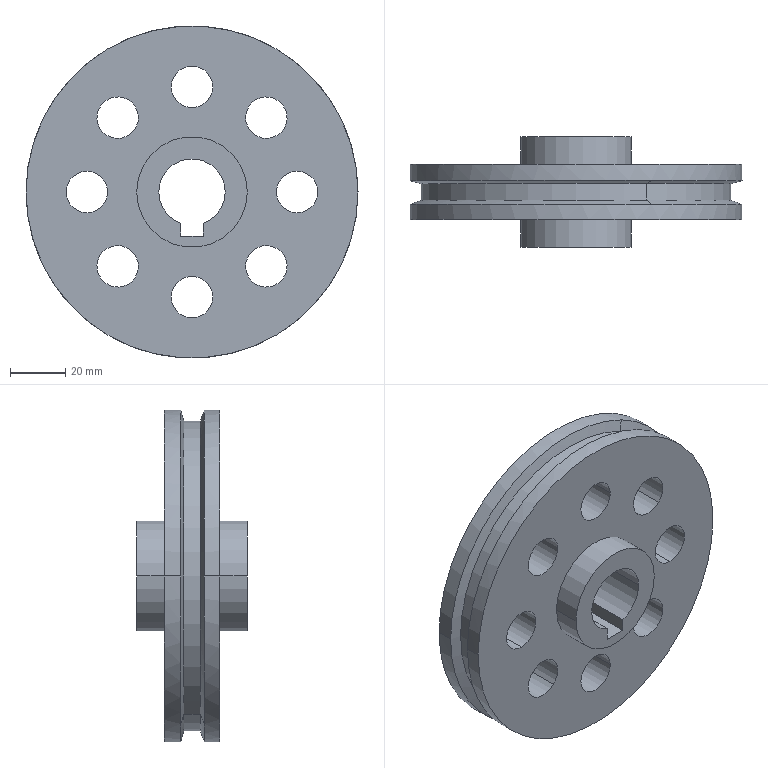Part | SolidWorks | 1 solid | 40 faces | box 120 x 40 x 120 mm | volume 192967 mm3 | cylinder 29 | plane 7 | cone 4 | commonest cylinder face diameters 15 x16 40 x4 120 x4 24 x3 112 x2
STEP:
#1=CARTESIAN_POINT('',(31.926,-178.476,-10.327));
#2=VERTEX_POINT('',#1);
#3=CARTESIAN_POINT('',(31.926,-158.476,-10.327));
#4=VERTEX_POINT('',#3);
#5=CARTESIAN_POINT('',(31.926,-178.476,-10.327));
#6=DIRECTION('',(0.,1.,0.));
#7=VECTOR('',#6,1000.);
#8=LINE('',#5,#7);
#9=EDGE_CURVE('',#2,#4,#8,.T.);
#10=ORIENTED_EDGE('',*,*,#9,.F.);
#11=CARTESIAN_POINT('',(42.533,-178.476,-20.933));
#12=VERTEX_POINT('',#11);
#13=CARTESIAN_POINT('',(37.229,-178.476,-15.63));
#14=DIRECTION('',(0.,-1.,0.));
#15=DIRECTION('',(-0.7071,0.,0.7071));
#16=AXIS2_PLACEMENT_3D('',#13,#14,#15);
#17=CIRCLE('',#16,7.5);
#18=EDGE_CURVE('',#2,#12,#17,.T.);
#19=ORIENTED_EDGE('',*,*,#18,.T.);
#20=CARTESIAN_POINT('',(42.533,-158.476,-20.933));
#21=VERTEX_POINT('',#20);
#22=CARTESIAN_POINT('',(42.533,-178.476,-20.933));
#23=DIRECTION('',(0.,1.,0.));
#24=VECTOR('',#23,1000.);
#25=LINE('',#22,#24);
#26=EDGE_CURVE('',#12,#21,#25,.T.);
#27=ORIENTED_EDGE('',*,*,#26,.T.);
#28=CARTESIAN_POINT('',(37.229,-158.476,-15.63));
#29=DIRECTION('',(0.,1.,0.));
#30=DIRECTION('',(0.7071,0.,-0.7071));
#31=AXIS2_PLACEMENT_3D('',#28,#29,#30);
#32=CIRCLE('',#31,7.5);
#33=EDGE_CURVE('',#21,#4,#32,.T.);
#34=ORIENTED_EDGE('',*,*,#33,.T.);
#35=EDGE_LOOP('',(#10,#19,#27,#34));
#36=FACE_OUTER_BOUND('',#35,.T.);
#37=CARTESIAN_POINT('',(37.229,-158.476,-15.63));
#38=DIRECTION('',(0.,1.,0.));
#39=DIRECTION('',(-0.7071,0.,0.7071));
#40=AXIS2_PLACEMENT_3D('',#37,#38,#39);
#41=CYLINDRICAL_SURFACE('',#40,7.5);
#42=ADVANCED_FACE('',(#36),#41,.F.);
#43=ORIENTED_EDGE('',*,*,#26,.F.);
#44=CARTESIAN_POINT('',(37.229,-178.476,-15.63));
#45=DIRECTION('',(0.,-1.,0.));
#46=DIRECTION('',(0.7071,0.,-0.7071));
#47=AXIS2_PLACEMENT_3D('',#44,#45,#46);
#48=CIRCLE('',#47,7.5);
#49=EDGE_CURVE('',#12,#2,#48,.T.);
#50=ORIENTED_EDGE('',*,*,#49,.T.);
#51=ORIENTED_EDGE('',*,*,#9,.T.);
#52=CARTESIAN_POINT('',(37.229,-158.476,-15.63));
#53=DIRECTION('',(0.,1.,0.));
#54=DIRECTION('',(-0.7071,0.,0.7071));
#55=AXIS2_PLACEMENT_3D('',#52,#53,#54);
#56=CIRCLE('',#55,7.5);
#57=EDGE_CURVE('',#4,#21,#56,.T.);
#58=ORIENTED_EDGE('',*,*,#57,.T.);
#59=EDGE_LOOP('',(#43,#50,#51,#58));
#60=FACE_OUTER_BOUND('',#59,.T.);
#61=CARTESIAN_POINT('',(37.229,-158.476,-15.63));
#62=DIRECTION('',(0.,1.,0.));
#63=DIRECTION('',(-0.7071,0.,0.7071));
#64=AXIS2_PLACEMENT_3D('',#61,#62,#63);
#65=CYLINDRICAL_SURFACE('',#64,7.5);
#66=ADVANCED_FACE('',(#60),#65,.F.);
#67=CARTESIAN_POINT('',(48.359,-178.476,-35.));
#68=VERTEX_POINT('',#67);
#69=CARTESIAN_POINT('',(48.359,-158.476,-35.));
#70=VERTEX_POINT('',#69);
#71=CARTESIAN_POINT('',(48.359,-178.476,-35.));
#72=DIRECTION('',(0.,1.,0.));
#73=VECTOR('',#72,1000.);
#74=LINE('',#71,#73);
#75=EDGE_CURVE('',#68,#70,#74,.T.);
#76=ORIENTED_EDGE('',*,*,#75,.F.);
#77=CARTESIAN_POINT('',(48.359,-178.476,-50.));
#78=VERTEX_POINT('',#77);
#79=CARTESIAN_POINT('',(48.359,-178.476,-42.5));
#80=DIRECTION('',(0.,-1.,0.));
#81=DIRECTION('',(0.,0.,1.));
#82=AXIS2_PLACEMENT_3D('',#79,#80,#81);
#83=CIRCLE('',#82,7.5);
#84=EDGE_CURVE('',#68,#78,#83,.T.);
#85=ORIENTED_EDGE('',*,*,#84,.T.);
#86=CARTESIAN_POINT('',(48.359,-158.476,-50.));
#87=VERTEX_POINT('',#86);
#88=CARTESIAN_POINT('',(48.359,-178.476,-50.));
#89=DIRECTION('',(0.,1.,0.));
#90=VECTOR('',#89,1000.);
#91=LINE('',#88,#90);
#92=EDGE_CURVE('',#78,#87,#91,.T.);
#93=ORIENTED_EDGE('',*,*,#92,.T.);
#94=CARTESIAN_POINT('',(48.359,-158.476,-42.5));
#95=DIRECTION('',(0.,1.,0.));
#96=DIRECTION('',(0.,0.,-1.));
#97=AXIS2_PLACEMENT_3D('',#94,#95,#96);
#98=CIRCLE('',#97,7.5);
#99=EDGE_CURVE('',#87,#70,#98,.T.);
#100=ORIENTED_EDGE('',*,*,#99,.T.);
#101=EDGE_LOOP('',(#76,#85,#93,#100));
#102=FACE_OUTER_BOUND('',#101,.T.);
#103=CARTESIAN_POINT('',(48.359,-158.476,-42.5));
#104=DIRECTION('',(0.,1.,0.));
#105=DIRECTION('',(0.,0.,1.));
#106=AXIS2_PLACEMENT_3D('',#103,#104,#105);
#107=CYLINDRICAL_SURFACE('',#106,7.5);
#108=ADVANCED_FACE('',(#102),#107,.F.);
#109=ORIENTED_EDGE('',*,*,#92,.F.);
#110=CARTESIAN_POINT('',(48.359,-178.476,-42.5));
#111=DIRECTION('',(0.,-1.,0.));
#112=DIRECTION('',(0.,0.,-1.));
#113=AXIS2_PLACEMENT_3D('',#110,#111,#112);
#114=CIRCLE('',#113,7.5);
#115=EDGE_CURVE('',#78,#68,#114,.T.);
#116=ORIENTED_EDGE('',*,*,#115,.T.);
#117=ORIENTED_EDGE('',*,*,#75,.T.);
#118=CARTESIAN_POINT('',(48.359,-158.476,-42.5));
#119=DIRECTION('',(0.,1.,0.));
#120=DIRECTION('',(0.,0.,1.));
#121=AXIS2_PLACEMENT_3D('',#118,#119,#120);
#122=CIRCLE('',#121,7.5);
#123=EDGE_CURVE('',#70,#87,#122,.T.);
#124=ORIENTED_EDGE('',*,*,#123,.T.);
#125=EDGE_LOOP('',(#109,#116,#117,#124));
#126=FACE_OUTER_BOUND('',#125,.T.);
#127=CARTESIAN_POINT('',(48.359,-158.476,-42.5));
#128=DIRECTION('',(0.,1.,0.));
#129=DIRECTION('',(0.,0.,1.));
#130=AXIS2_PLACEMENT_3D('',#127,#128,#129);
#131=CYLINDRICAL_SURFACE('',#130,7.5);
#132=ADVANCED_FACE('',(#126),#131,.F.);
#133=CARTESIAN_POINT('',(42.533,-178.476,-64.067));
#134=VERTEX_POINT('',#133);
#135=CARTESIAN_POINT('',(42.533,-158.476,-64.067));
#136=VERTEX_POINT('',#135);
#137=CARTESIAN_POINT('',(42.533,-178.476,-64.067));
#138=DIRECTION('',(0.,1.,0.));
#139=VECTOR('',#138,1000.);
#140=LINE('',#137,#139);
#141=EDGE_CURVE('',#134,#136,#140,.T.);
#142=ORIENTED_EDGE('',*,*,#141,.F.);
#143=CARTESIAN_POINT('',(31.926,-178.476,-74.673));
#144=VERTEX_POINT('',#143);
#145=CARTESIAN_POINT('',(37.229,-178.476,-69.37));
#146=DIRECTION('',(0.,-1.,0.));
#147=DIRECTION('',(0.7071,0.,0.7071));
#148=AXIS2_PLACEMENT_3D('',#145,#146,#147);
#149=CIRCLE('',#148,7.5);
#150=EDGE_CURVE('',#134,#144,#149,.T.);
#151=ORIENTED_EDGE('',*,*,#150,.T.);
#152=CARTESIAN_POINT('',(31.926,-158.476,-74.673));
#153=VERTEX_POINT('',#152);
#154=CARTESIAN_POINT('',(31.926,-178.476,-74.673));
#155=DIRECTION('',(0.,1.,0.));
#156=VECTOR('',#155,1000.);
#157=LINE('',#154,#156);
#158=EDGE_CURVE('',#144,#153,#157,.T.);
#159=ORIENTED_EDGE('',*,*,#158,.T.);
#160=CARTESIAN_POINT('',(37.229,-158.476,-69.37));
#161=DIRECTION('',(0.,1.,0.));
#162=DIRECTION('',(-0.7071,0.,-0.7071));
#163=AXIS2_PLACEMENT_3D('',#160,#161,#162);
#164=CIRCLE('',#163,7.5);
#165=EDGE_CURVE('',#153,#136,#164,.T.);
#166=ORIENTED_EDGE('',*,*,#165,.T.);
#167=EDGE_LOOP('',(#142,#151,#159,#166));
#168=FACE_OUTER_BOUND('',#167,.T.);
#169=CARTESIAN_POINT('',(37.229,-158.476,-69.37));
#170=DIRECTION('',(0.,1.,0.));
#171=DIRECTION('',(0.7071,0.,0.7071));
#172=AXIS2_PLACEMENT_3D('',#169,#170,#171);
#173=CYLINDRICAL_SURFACE('',#172,7.5);
#174=ADVANCED_FACE('',(#168),#173,.F.);
#175=ORIENTED_EDGE('',*,*,#158,.F.);
#176=CARTESIAN_POINT('',(37.229,-178.476,-69.37));
#177=DIRECTION('',(0.,-1.,0.));
#178=DIRECTION('',(-0.7071,0.,-0.7071));
#179=AXIS2_PLACEMENT_3D('',#176,#177,#178);
#180=CIRCLE('',#179,7.5);
#181=EDGE_CURVE('',#144,#134,#180,.T.);
#182=ORIENTED_EDGE('',*,*,#181,.T.);
#183=ORIENTED_EDGE('',*,*,#141,.T.);
#184=CARTESIAN_POINT('',(37.229,-158.476,-69.37));
#185=DIRECTION('',(0.,1.,0.));
#186=DIRECTION('',(0.7071,0.,0.7071));
#187=AXIS2_PLACEMENT_3D('',#184,#185,#186);
#188=CIRCLE('',#187,7.5);
#189=EDGE_CURVE('',#136,#153,#188,.T.);
#190=ORIENTED_EDGE('',*,*,#189,.T.);
#191=EDGE_LOOP('',(#175,#182,#183,#190));
#192=FACE_OUTER_BOUND('',#191,.T.);
#193=CARTESIAN_POINT('',(37.229,-158.476,-69.37));
#194=DIRECTION('',(0.,1.,0.));
#195=DIRECTION('',(0.7071,0.,0.7071));
#196=AXIS2_PLACEMENT_3D('',#193,#194,#195);
#197=CYLINDRICAL_SURFACE('',#196,7.5);
#198=ADVANCED_FACE('',(#192),#197,.F.);
#199=CARTESIAN_POINT('',(17.859,-178.476,-80.5));
#200=VERTEX_POINT('',#199);
#201=CARTESIAN_POINT('',(17.859,-158.476,-80.5));
#202=VERTEX_POINT('',#201);
#203=CARTESIAN_POINT('',(17.859,-178.476,-80.5));
#204=DIRECTION('',(0.,1.,0.));
#205=VECTOR('',#204,1000.);
#206=LINE('',#203,#205);
#207=EDGE_CURVE('',#200,#202,#206,.T.);
#208=ORIENTED_EDGE('',*,*,#207,.F.);
#209=CARTESIAN_POINT('',(2.859,-178.476,-80.5));
#210=VERTEX_POINT('',#209);
#211=CARTESIAN_POINT('',(10.359,-178.476,-80.5));
#212=DIRECTION('',(0.,-1.,0.));
#213=DIRECTION('',(1.,0.,0.));
#214=AXIS2_PLACEMENT_3D('',#211,#212,#213);
#215=CIRCLE('',#214,7.5);
#216=EDGE_CURVE('',#200,#210,#215,.T.);
#217=ORIENTED_EDGE('',*,*,#216,.T.);
#218=CARTESIAN_POINT('',(2.859,-158.476,-80.5));
#219=VERTEX_POINT('',#218);
#220=CARTESIAN_POINT('',(2.859,-178.476,-80.5));
#221=DIRECTION('',(0.,1.,0.));
#222=VECTOR('',#221,1000.);
#223=LINE('',#220,#222);
#224=EDGE_CURVE('',#210,#219,#223,.T.);
#225=ORIENTED_EDGE('',*,*,#224,.T.);
#226=CARTESIAN_POINT('',(10.359,-158.476,-80.5));
#227=DIRECTION('',(0.,1.,0.));
#228=DIRECTION('',(-1.,0.,0.));
#229=AXIS2_PLACEMENT_3D('',#226,#227,#228);
#230=CIRCLE('',#229,7.5);
#231=EDGE_CURVE('',#219,#202,#230,.T.);
#232=ORIENTED_EDGE('',*,*,#231,.T.);
#233=EDGE_LOOP('',(#208,#217,#225,#232));
#234=FACE_OUTER_BOUND('',#233,.T.);
#235=CARTESIAN_POINT('',(10.359,-158.476,-80.5));
#236=DIRECTION('',(0.,1.,0.));
#237=DIRECTION('',(1.,0.,0.));
#238=AXIS2_PLACEMENT_3D('',#235,#236,#237);
#239=CYLINDRICAL_SURFACE('',#238,7.5);
#240=ADVANCED_FACE('',(#234),#239,.F.);
#241=ORIENTED_EDGE('',*,*,#224,.F.);
#242=CARTESIAN_POINT('',(10.359,-178.476,-80.5));
#243=DIRECTION('',(0.,-1.,0.));
#244=DIRECTION('',(-1.,0.,0.));
#245=AXIS2_PLACEMENT_3D('',#242,#243,#244);
#246=CIRCLE('',#245,7.5);
#247=EDGE_CURVE('',#210,#200,#246,.T.);
#248=ORIENTED_EDGE('',*,*,#247,.T.);
#249=ORIENTED_EDGE('',*,*,#207,.T.);
#250=CARTESIAN_POINT('',(10.359,-158.476,-80.5));
#251=DIRECTION('',(0.,1.,0.));
#252=DIRECTION('',(1.,0.,0.));
#253=AXIS2_PLACEMENT_3D('',#250,#251,#252);
#254=CIRCLE('',#253,7.5);
#255=EDGE_CURVE('',#202,#219,#254,.T.);
#256=ORIENTED_EDGE('',*,*,#255,.T.);
#257=EDGE_LOOP('',(#241,#248,#249,#256));
#258=FACE_OUTER_BOUND('',#257,.T.);
#259=CARTESIAN_POINT('',(10.359,-158.476,-80.5));
#260=DIRECTION('',(0.,1.,0.));
#261=DIRECTION('',(1.,0.,0.));
#262=AXIS2_PLACEMENT_3D('',#259,#260,#261);
#263=CYLINDRICAL_SURFACE('',#262,7.5);
#264=ADVANCED_FACE('',(#258),#263,.F.);
#265=CARTESIAN_POINT('',(-11.207,-178.476,-74.673));
#266=VERTEX_POINT('',#265);
#267=CARTESIAN_POINT('',(-11.207,-158.476,-74.673));
#268=VERTEX_POINT('',#267);
#269=CARTESIAN_POINT('',(-11.207,-178.476,-74.673));
#270=DIRECTION('',(0.,1.,0.));
#271=VECTOR('',#270,1000.);
#272=LINE('',#269,#271);
#273=EDGE_CURVE('',#266,#268,#272,.T.);
#274=ORIENTED_EDGE('',*,*,#273,.F.);
#275=CARTESIAN_POINT('',(-21.814,-178.476,-64.067));
#276=VERTEX_POINT('',#275);
#277=CARTESIAN_POINT('',(-16.511,-178.476,-69.37));
#278=DIRECTION('',(0.,-1.,0.));
#279=DIRECTION('',(0.7071,0.,-0.7071));
#280=AXIS2_PLACEMENT_3D('',#277,#278,#279);
#281=CIRCLE('',#280,7.5);
#282=EDGE_CURVE('',#266,#276,#281,.T.);
#283=ORIENTED_EDGE('',*,*,#282,.T.);
#284=CARTESIAN_POINT('',(-21.814,-158.476,-64.067));
#285=VERTEX_POINT('',#284);
#286=CARTESIAN_POINT('',(-21.814,-178.476,-64.067));
#287=DIRECTION('',(0.,1.,0.));
#288=VECTOR('',#287,1000.);
#289=LINE('',#286,#288);
#290=EDGE_CURVE('',#276,#285,#289,.T.);
#291=ORIENTED_EDGE('',*,*,#290,.T.);
#292=CARTESIAN_POINT('',(-16.511,-158.476,-69.37));
#293=DIRECTION('',(0.,1.,0.));
#294=DIRECTION('',(-0.7071,0.,0.7071));
#295=AXIS2_PLACEMENT_3D('',#292,#293,#294);
#296=CIRCLE('',#295,7.5);
#297=EDGE_CURVE('',#285,#268,#296,.T.);
#298=ORIENTED_EDGE('',*,*,#297,.T.);
#299=EDGE_LOOP('',(#274,#283,#291,#298));
#300=FACE_OUTER_BOUND('',#299,.T.);
#301=CARTESIAN_POINT('',(-16.511,-158.476,-69.37));
#302=DIRECTION('',(0.,1.,0.));
#303=DIRECTION('',(0.7071,0.,-0.7071));
#304=AXIS2_PLACEMENT_3D('',#301,#302,#303);
#305=CYLINDRICAL_SURFACE('',#304,7.5);
#306=ADVANCED_FACE('',(#300),#305,.F.);
#307=ORIENTED_EDGE('',*,*,#290,.F.);
#308=CARTESIAN_POINT('',(-16.511,-178.476,-69.37));
#309=DIRECTION('',(0.,-1.,0.));
#310=DIRECTION('',(-0.7071,0.,0.7071));
#311=AXIS2_PLACEMENT_3D('',#308,#309,#310);
#312=CIRCLE('',#311,7.5);
#313=EDGE_CURVE('',#276,#266,#312,.T.);
#314=ORIENTED_EDGE('',*,*,#313,.T.);
#315=ORIENTED_EDGE('',*,*,#273,.T.);
#316=CARTESIAN_POINT('',(-16.511,-158.476,-69.37));
#317=DIRECTION('',(0.,1.,0.));
#318=DIRECTION('',(0.7071,0.,-0.7071));
#319=AXIS2_PLACEMENT_3D('',#316,#317,#318);
#320=CIRCLE('',#319,7.5);
#321=EDGE_CURVE('',#268,#285,#320,.T.);
#322=ORIENTED_EDGE('',*,*,#321,.T.);
#323=EDGE_LOOP('',(#307,#314,#315,#322));
#324=FACE_OUTER_BOUND('',#323,.T.);
#325=CARTESIAN_POINT('',(-16.511,-158.476,-69.37));
#326=DIRECTION('',(0.,1.,0.));
#327=DIRECTION('',(0.7071,0.,-0.7071));
#328=AXIS2_PLACEMENT_3D('',#325,#326,#327);
#329=CYLINDRICAL_SURFACE('',#328,7.5);
#330=ADVANCED_FACE('',(#324),#329,.F.);
#331=CARTESIAN_POINT('',(-27.641,-178.476,-50.));
#332=VERTEX_POINT('',#331);
#333=CARTESIAN_POINT('',(-27.641,-158.476,-50.));
#334=VERTEX_POINT('',#333);
#335=CARTESIAN_POINT('',(-27.641,-178.476,-50.));
#336=DIRECTION('',(0.,1.,0.));
#337=VECTOR('',#336,1000.);
#338=LINE('',#335,#337);
#339=EDGE_CURVE('',#332,#334,#338,.T.);
#340=ORIENTED_EDGE('',*,*,#339,.F.);
#341=CARTESIAN_POINT('',(-27.641,-178.476,-35.));
#342=VERTEX_POINT('',#341);
#343=CARTESIAN_POINT('',(-27.641,-178.476,-42.5));
#344=DIRECTION('',(0.,-1.,0.));
#345=DIRECTION('',(0.,0.,-1.));
#346=AXIS2_PLACEMENT_3D('',#343,#344,#345);
#347=CIRCLE('',#346,7.5);
#348=EDGE_CURVE('',#332,#342,#347,.T.);
#349=ORIENTED_EDGE('',*,*,#348,.T.);
#350=CARTESIAN_POINT('',(-27.641,-158.476,-35.));
#351=VERTEX_POINT('',#350);
#352=CARTESIAN_POINT('',(-27.641,-178.476,-35.));
#353=DIRECTION('',(0.,1.,0.));
#354=VECTOR('',#353,1000.);
#355=LINE('',#352,#354);
#356=EDGE_CURVE('',#342,#351,#355,.T.);
#357=ORIENTED_EDGE('',*,*,#356,.T.);
#358=CARTESIAN_POINT('',(-27.641,-158.476,-42.5));
#359=DIRECTION('',(0.,1.,0.));
#360=DIRECTION('',(0.,0.,1.));
#361=AXIS2_PLACEMENT_3D('',#358,#359,#360);
#362=CIRCLE('',#361,7.5);
#363=EDGE_CURVE('',#351,#334,#362,.T.);
#364=ORIENTED_EDGE('',*,*,#363,.T.);
#365=EDGE_LOOP('',(#340,#349,#357,#364));
#366=FACE_OUTER_BOUND('',#365,.T.);
#367=CARTESIAN_POINT('',(-27.641,-158.476,-42.5));
#368=DIRECTION('',(0.,1.,0.));
#369=DIRECTION('',(0.,0.,-1.));
#370=AXIS2_PLACEMENT_3D('',#367,#368,#369);
#371=CYLINDRICAL_SURFACE('',#370,7.5);
#372=ADVANCED_FACE('',(#366),#371,.F.);
#373=ORIENTED_EDGE('',*,*,#356,.F.);
#374=CARTESIAN_POINT('',(-27.641,-178.476,-42.5));
#375=DIRECTION('',(0.,-1.,0.));
#376=DIRECTION('',(0.,0.,1.));
#377=AXIS2_PLACEMENT_3D('',#374,#375,#376);
#378=CIRCLE('',#377,7.5);
#379=EDGE_CURVE('',#342,#332,#378,.T.);
#380=ORIENTED_EDGE('',*,*,#379,.T.);
#381=ORIENTED_EDGE('',*,*,#339,.T.);
#382=CARTESIAN_POINT('',(-27.641,-158.476,-42.5));
#383=DIRECTION('',(0.,1.,0.));
#384=DIRECTION('',(0.,0.,-1.));
#385=AXIS2_PLACEMENT_3D('',#382,#383,#384);
#386=CIRCLE('',#385,7.5);
#387=EDGE_CURVE('',#334,#351,#386,.T.);
#388=ORIENTED_EDGE('',*,*,#387,.T.);
#389=EDGE_LOOP('',(#373,#380,#381,#388));
#390=FACE_OUTER_BOUND('',#389,.T.);
#391=CARTESIAN_POINT('',(-27.641,-158.476,-42.5));
#392=DIRECTION('',(0.,1.,0.));
#393=DIRECTION('',(0.,0.,-1.));
#394=AXIS2_PLACEMENT_3D('',#391,#392,#393);
#395=CYLINDRICAL_SURFACE('',#394,7.5);
#396=ADVANCED_FACE('',(#390),#395,.F.);
#397=CARTESIAN_POINT('',(-21.814,-178.476,-20.933));
#398=VERTEX_POINT('',#397);
#399=CARTESIAN_POINT('',(-21.814,-158.476,-20.933));
#400=VERTEX_POINT('',#399);
#401=CARTESIAN_POINT('',(-21.814,-178.476,-20.933));
#402=DIRECTION('',(0.,1.,0.));
#403=VECTOR('',#402,1000.);
#404=LINE('',#401,#403);
#405=EDGE_CURVE('',#398,#400,#404,.T.);
#406=ORIENTED_EDGE('',*,*,#405,.F.);
#407=CARTESIAN_POINT('',(-11.207,-178.476,-10.327));
#408=VERTEX_POINT('',#407);
#409=CARTESIAN_POINT('',(-16.511,-178.476,-15.63));
#410=DIRECTION('',(0.,-1.,0.));
#411=DIRECTION('',(-0.7071,0.,-0.7071));
#412=AXIS2_PLACEMENT_3D('',#409,#410,#411);
#413=CIRCLE('',#412,7.5);
#414=EDGE_CURVE('',#398,#408,#413,.T.);
#415=ORIENTED_EDGE('',*,*,#414,.T.);
#416=CARTESIAN_POINT('',(-11.207,-158.476,-10.327));
#417=VERTEX_POINT('',#416);
#418=CARTESIAN_POINT('',(-11.207,-178.476,-10.327));
#419=DIRECTION('',(0.,1.,0.));
#420=VECTOR('',#419,1000.);
#421=LINE('',#418,#420);
#422=EDGE_CURVE('',#408,#417,#421,.T.);
#423=ORIENTED_EDGE('',*,*,#422,.T.);
#424=CARTESIAN_POINT('',(-16.511,-158.476,-15.63));
#425=DIRECTION('',(0.,1.,0.));
#426=DIRECTION('',(0.7071,0.,0.7071));
#427=AXIS2_PLACEMENT_3D('',#424,#425,#426);
#428=CIRCLE('',#427,7.5);
#429=EDGE_CURVE('',#417,#400,#428,.T.);
#430=ORIENTED_EDGE('',*,*,#429,.T.);
#431=EDGE_LOOP('',(#406,#415,#423,#430));
#432=FACE_OUTER_BOUND('',#431,.T.);
#433=CARTESIAN_POINT('',(-16.511,-158.476,-15.63));
#434=DIRECTION('',(0.,1.,0.));
#435=DIRECTION('',(-0.7071,0.,-0.7071));
#436=AXIS2_PLACEMENT_3D('',#433,#434,#435);
#437=CYLINDRICAL_SURFACE('',#436,7.5);
#438=ADVANCED_FACE('',(#432),#437,.F.);
#439=ORIENTED_EDGE('',*,*,#422,.F.);
#440=CARTESIAN_POINT('',(-16.511,-178.476,-15.63));
#441=DIRECTION('',(0.,-1.,0.));
#442=DIRECTION('',(0.7071,0.,0.7071));
#443=AXIS2_PLACEMENT_3D('',#440,#441,#442);
#444=CIRCLE('',#443,7.5);
#445=EDGE_CURVE('',#408,#398,#444,.T.);
#446=ORIENTED_EDGE('',*,*,#445,.T.);
#447=ORIENTED_EDGE('',*,*,#405,.T.);
#448=CARTESIAN_POINT('',(-16.511,-158.476,-15.63));
#449=DIRECTION('',(0.,1.,0.));
#450=DIRECTION('',(-0.7071,0.,-0.7071));
#451=AXIS2_PLACEMENT_3D('',#448,#449,#450);
#452=CIRCLE('',#451,7.5);
#453=EDGE_CURVE('',#400,#417,#452,.T.);
#454=ORIENTED_EDGE('',*,*,#453,.T.);
#455=EDGE_LOOP('',(#439,#446,#447,#454));
#456=FACE_OUTER_BOUND('',#455,.T.);
#457=CARTESIAN_POINT('',(-16.511,-158.476,-15.63));
#458=DIRECTION('',(0.,1.,0.));
#459=DIRECTION('',(-0.7071,0.,-0.7071));
#460=AXIS2_PLACEMENT_3D('',#457,#458,#459);
#461=CYLINDRICAL_SURFACE('',#460,7.5);
#462=ADVANCED_FACE('',(#456),#461,.F.);
#463=CARTESIAN_POINT('',(2.859,-178.476,-4.5));
#464=VERTEX_POINT('',#463);
#465=CARTESIAN_POINT('',(2.859,-158.476,-4.5));
#466=VERTEX_POINT('',#465);
#467=CARTESIAN_POINT('',(2.859,-178.476,-4.5));
#468=DIRECTION('',(0.,1.,0.));
#469=VECTOR('',#468,1000.);
#470=LINE('',#467,#469);
#471=EDGE_CURVE('',#464,#466,#470,.T.);
#472=ORIENTED_EDGE('',*,*,#471,.F.);
#473=CARTESIAN_POINT('',(17.859,-178.476,-4.5));
#474=VERTEX_POINT('',#473);
#475=CARTESIAN_POINT('',(10.359,-178.476,-4.5));
#476=DIRECTION('',(0.,-1.,0.));
#477=DIRECTION('',(-1.,0.,0.));
#478=AXIS2_PLACEMENT_3D('',#475,#476,#477);
#479=CIRCLE('',#478,7.5);
#480=EDGE_CURVE('',#464,#474,#479,.T.);
#481=ORIENTED_EDGE('',*,*,#480,.T.);
#482=CARTESIAN_POINT('',(17.859,-158.476,-4.5));
#483=VERTEX_POINT('',#482);
#484=CARTESIAN_POINT('',(17.859,-178.476,-4.5));
#485=DIRECTION('',(0.,1.,0.));
#486=VECTOR('',#485,1000.);
#487=LINE('',#484,#486);
#488=EDGE_CURVE('',#474,#483,#487,.T.);
#489=ORIENTED_EDGE('',*,*,#488,.T.);
#490=CARTESIAN_POINT('',(10.359,-158.476,-4.5));
#491=DIRECTION('',(0.,1.,0.));
#492=DIRECTION('',(1.,0.,0.));
#493=AXIS2_PLACEMENT_3D('',#490,#491,#492);
#494=CIRCLE('',#493,7.5);
#495=EDGE_CURVE('',#483,#466,#494,.T.);
#496=ORIENTED_EDGE('',*,*,#495,.T.);
#497=EDGE_LOOP('',(#472,#481,#489,#496));
#498=FACE_OUTER_BOUND('',#497,.T.);
#499=CARTESIAN_POINT('',(10.359,-158.476,-4.5));
#500=DIRECTION('',(0.,1.,0.));
#501=DIRECTION('',(-1.,0.,0.));
#502=AXIS2_PLACEMENT_3D('',#499,#500,#501);
#503=CYLINDRICAL_SURFACE('',#502,7.5);
#504=ADVANCED_FACE('',(#498),#503,.F.);
#505=ORIENTED_EDGE('',*,*,#488,.F.);
#506=CARTESIAN_POINT('',(10.359,-178.476,-4.5));
#507=DIRECTION('',(0.,-1.,0.));
#508=DIRECTION('',(1.,0.,0.));
#509=AXIS2_PLACEMENT_3D('',#506,#507,#508);
#510=CIRCLE('',#509,7.5);
#511=EDGE_CURVE('',#474,#464,#510,.T.);
#512=ORIENTED_EDGE('',*,*,#511,.T.);
#513=ORIENTED_EDGE('',*,*,#471,.T.);
#514=CARTESIAN_POINT('',(10.359,-158.476,-4.5));
#515=DIRECTION('',(0.,1.,0.));
#516=DIRECTION('',(-1.,0.,0.));
#517=AXIS2_PLACEMENT_3D('',#514,#515,#516);
#518=CIRCLE('',#517,7.5);
#519=EDGE_CURVE('',#466,#483,#518,.T.);
#520=ORIENTED_EDGE('',*,*,#519,.T.);
#521=EDGE_LOOP('',(#505,#512,#513,#520));
#522=FACE_OUTER_BOUND('',#521,.T.);
#523=CARTESIAN_POINT('',(10.359,-158.476,-4.5));
#524=DIRECTION('',(0.,1.,0.));
#525=DIRECTION('',(-1.,0.,0.));
#526=AXIS2_PLACEMENT_3D('',#523,#524,#525);
#527=CYLINDRICAL_SURFACE('',#526,7.5);
#528=ADVANCED_FACE('',(#522),#527,.F.);
#529=CARTESIAN_POINT('',(-1.641,-148.476,-42.5));
#530=VERTEX_POINT('',#529);
#531=CARTESIAN_POINT('',(22.359,-148.476,-42.5));
#532=VERTEX_POINT('',#531);
#533=CARTESIAN_POINT('',(10.359,-148.476,-42.5));
#534=DIRECTION('',(0.,1.,0.));
#535=DIRECTION('',(-1.,0.,0.));
#536=AXIS2_PLACEMENT_3D('',#533,#534,#535);
#537=CIRCLE('',#536,12.);
#538=EDGE_CURVE('',#530,#532,#537,.T.);
#539=ORIENTED_EDGE('',*,*,#538,.T.);
#540=CARTESIAN_POINT('',(22.359,-188.476,-42.5));
#541=VERTEX_POINT('',#540);
#542=CARTESIAN_POINT('',(22.359,-188.476,-42.5));
#543=DIRECTION('',(0.,1.,0.));
#544=VECTOR('',#543,1000.);
#545=LINE('',#542,#544);
#546=EDGE_CURVE('',#541,#532,#545,.T.);
#547=ORIENTED_EDGE('',*,*,#546,.F.);
#548=CARTESIAN_POINT('',(-1.641,-188.476,-42.5));
#549=VERTEX_POINT('',#548);
#550=CARTESIAN_POINT('',(10.359,-188.476,-42.5));
#551=DIRECTION('',(0.,-1.,0.));
#552=DIRECTION('',(1.,0.,0.));
#553=AXIS2_PLACEMENT_3D('',#550,#551,#552);
#554=CIRCLE('',#553,12.);
#555=EDGE_CURVE('',#541,#549,#554,.T.);
#556=ORIENTED_EDGE('',*,*,#555,.T.);
#557=CARTESIAN_POINT('',(-1.641,-188.476,-42.5));
#558=DIRECTION('',(0.,1.,0.));
#559=VECTOR('',#558,1000.);
#560=LINE('',#557,#559);
#561=EDGE_CURVE('',#549,#530,#560,.T.);
#562=ORIENTED_EDGE('',*,*,#561,.T.);
#563=EDGE_LOOP('',(#539,#547,#556,#562));
#564=FACE_OUTER_BOUND('',#563,.T.);
#565=CARTESIAN_POINT('',(10.359,-148.476,-42.5));
#566=DIRECTION('',(0.,-1.,0.));
#567=DIRECTION('',(1.,0.,0.));
#568=AXIS2_PLACEMENT_3D('',#565,#566,#567);
#569=CYLINDRICAL_SURFACE('',#568,12.);
#570=ADVANCED_FACE('',(#564),#569,.F.);
#571=CARTESIAN_POINT('',(14.359,-148.476,-53.814));
#572=VERTEX_POINT('',#571);
#573=CARTESIAN_POINT('',(10.359,-148.476,-42.5));
#574=DIRECTION('',(0.,1.,0.));
#575=DIRECTION('',(1.,0.,0.));
#576=AXIS2_PLACEMENT_3D('',#573,#574,#575);
#577=CIRCLE('',#576,12.);
#578=EDGE_CURVE('',#532,#572,#577,.T.);
#579=ORIENTED_EDGE('',*,*,#578,.T.);
#580=CARTESIAN_POINT('',(14.359,-188.476,-53.814));
#581=VERTEX_POINT('',#580);
#582=CARTESIAN_POINT('',(14.359,-188.476,-53.814));
#583=DIRECTION('',(0.,1.,0.));
#584=VECTOR('',#583,1000.);
#585=LINE('',#582,#584);
#586=EDGE_CURVE('',#581,#572,#585,.T.);
#587=ORIENTED_EDGE('',*,*,#586,.F.);
#588=CARTESIAN_POINT('',(10.359,-188.476,-42.5));
#589=DIRECTION('',(0.,-1.,0.));
#590=DIRECTION('',(0.3333,0.,-0.9428));
#591=AXIS2_PLACEMENT_3D('',#588,#589,#590);
#592=CIRCLE('',#591,12.);
#593=EDGE_CURVE('',#581,#541,#592,.T.);
#594=ORIENTED_EDGE('',*,*,#593,.T.);
#595=ORIENTED_EDGE('',*,*,#546,.T.);
#596=EDGE_LOOP('',(#579,#587,#594,#595));
#597=FACE_OUTER_BOUND('',#596,.T.);
#598=CARTESIAN_POINT('',(10.359,-148.476,-42.5));
#599=DIRECTION('',(0.,-1.,0.));
#600=DIRECTION('',(1.,0.,0.));
#601=AXIS2_PLACEMENT_3D('',#598,#599,#600);
#602=CYLINDRICAL_SURFACE('',#601,12.);
#603=ADVANCED_FACE('',(#597),#602,.F.);
#604=CARTESIAN_POINT('',(14.359,-188.476,-58.496));
#605=VERTEX_POINT('',#604);
#606=CARTESIAN_POINT('',(14.359,-188.476,-53.814));
#607=DIRECTION('',(0.,0.,-1.));
#608=VECTOR('',#607,1000.);
#609=LINE('',#606,#608);
#610=EDGE_CURVE('',#581,#605,#609,.T.);
#611=ORIENTED_EDGE('',*,*,#610,.F.);
#612=ORIENTED_EDGE('',*,*,#586,.T.);
#613=CARTESIAN_POINT('',(14.359,-148.476,-58.496));
#614=VERTEX_POINT('',#613);
#615=CARTESIAN_POINT('',(14.359,-148.476,-53.814));
#616=DIRECTION('',(0.,0.,-1.));
#617=VECTOR('',#616,1000.);
#618=LINE('',#615,#617);
#619=EDGE_CURVE('',#572,#614,#618,.T.);
#620=ORIENTED_EDGE('',*,*,#619,.T.);
#621=CARTESIAN_POINT('',(14.359,-148.476,-58.496));
#622=DIRECTION('',(0.,-1.,0.));
#623=VECTOR('',#622,1000.);
#624=LINE('',#621,#623);
#625=EDGE_CURVE('',#614,#605,#624,.T.);
#626=ORIENTED_EDGE('',*,*,#625,.T.);
#627=EDGE_LOOP('',(#611,#612,#620,#626));
#628=FACE_OUTER_BOUND('',#627,.T.);
#629=CARTESIAN_POINT('',(14.359,-188.476,-58.496));
#630=DIRECTION('',(1.,0.,0.));
#631=DIRECTION('',(0.,1.,0.));
#632=AXIS2_PLACEMENT_3D('',#629,#630,#631);
#633=PLANE('',#632);
#634=ADVANCED_FACE('',(#628),#633,.F.);
#635=CARTESIAN_POINT('',(6.359,-188.476,-53.814));
#636=VERTEX_POINT('',#635);
#637=CARTESIAN_POINT('',(10.359,-188.476,-42.5));
#638=DIRECTION('',(0.,-1.,0.));
#639=DIRECTION('',(-1.,0.,0.));
#640=AXIS2_PLACEMENT_3D('',#637,#638,#639);
#641=CIRCLE('',#640,12.);
#642=EDGE_CURVE('',#549,#636,#641,.T.);
#643=ORIENTED_EDGE('',*,*,#642,.F.);
#644=ORIENTED_EDGE('',*,*,#555,.F.);
#645=ORIENTED_EDGE('',*,*,#593,.F.);
#646=ORIENTED_EDGE('',*,*,#610,.T.);
#647=CARTESIAN_POINT('',(6.359,-188.476,-58.496));
#648=VERTEX_POINT('',#647);
#649=CARTESIAN_POINT('',(14.359,-188.476,-58.496));
#650=DIRECTION('',(-1.,0.,0.));
#651=VECTOR('',#650,1000.);
#652=LINE('',#649,#651);
#653=EDGE_CURVE('',#605,#648,#652,.T.);
#654=ORIENTED_EDGE('',*,*,#653,.T.);
#655=CARTESIAN_POINT('',(6.359,-188.476,-58.496));
#656=DIRECTION('',(0.,0.,1.));
#657=VECTOR('',#656,1000.);
#658=LINE('',#655,#657);
#659=EDGE_CURVE('',#648,#636,#658,.T.);
#660=ORIENTED_EDGE('',*,*,#659,.T.);
#661=EDGE_LOOP('',(#643,#644,#645,#646,#654,#660));
#662=FACE_BOUND('',#661,.T.);
#663=CARTESIAN_POINT('',(-9.641,-188.476,-42.5));
#664=VERTEX_POINT('',#663);
#665=CARTESIAN_POINT('',(30.359,-188.476,-42.5));
#666=VERTEX_POINT('',#665);
#667=CARTESIAN_POINT('',(10.359,-188.476,-42.5));
#668=DIRECTION('',(0.,1.,0.));
#669=DIRECTION('',(-1.,0.,0.));
#670=AXIS2_PLACEMENT_3D('',#667,#668,#669);
#671=CIRCLE('',#670,20.);
#672=EDGE_CURVE('',#664,#666,#671,.T.);
#673=ORIENTED_EDGE('',*,*,#672,.F.);
#674=CARTESIAN_POINT('',(10.359,-188.476,-42.5));
#675=DIRECTION('',(0.,1.,0.));
#676=DIRECTION('',(1.,0.,0.));
#677=AXIS2_PLACEMENT_3D('',#674,#675,#676);
#678=CIRCLE('',#677,20.);
#679=EDGE_CURVE('',#666,#664,#678,.T.);
#680=ORIENTED_EDGE('',*,*,#679,.F.);
#681=EDGE_LOOP('',(#673,#680));
#682=FACE_OUTER_BOUND('',#681,.T.);
#683=CARTESIAN_POINT('',(0.,-188.476,0.));
#684=DIRECTION('',(0.,-1.,0.));
#685=DIRECTION('',(0.,0.,-1.));
#686=AXIS2_PLACEMENT_3D('',#683,#684,#685);
#687=PLANE('',#686);
#688=ADVANCED_FACE('',(#662,#682),#687,.T.);
#689=ORIENTED_EDGE('',*,*,#672,.T.);
#690=CARTESIAN_POINT('',(30.359,-178.476,-42.5));
#691=VERTEX_POINT('',#690);
#692=CARTESIAN_POINT('',(30.359,-188.476,-42.5));
#693=DIRECTION('',(0.,1.,0.));
#694=VECTOR('',#693,1000.);
#695=LINE('',#692,#694);
#696=EDGE_CURVE('',#666,#691,#695,.T.);
#697=ORIENTED_EDGE('',*,*,#696,.T.);
#698=CARTESIAN_POINT('',(-9.641,-178.476,-42.5));
#699=VERTEX_POINT('',#698);
#700=CARTESIAN_POINT('',(10.359,-178.476,-42.5));
#701=DIRECTION('',(0.,-1.,0.));
#702=DIRECTION('',(1.,0.,0.));
#703=AXIS2_PLACEMENT_3D('',#700,#701,#702);
#704=CIRCLE('',#703,20.);
#705=EDGE_CURVE('',#691,#699,#704,.T.);
#706=ORIENTED_EDGE('',*,*,#705,.T.);
#707=CARTESIAN_POINT('',(-9.641,-188.476,-42.5));
#708=DIRECTION('',(0.,1.,0.));
#709=VECTOR('',#708,1000.);
#710=LINE('',#707,#709);
#711=EDGE_CURVE('',#664,#699,#710,.T.);
#712=ORIENTED_EDGE('',*,*,#711,.F.);
#713=EDGE_LOOP('',(#689,#697,#706,#712));
#714=FACE_OUTER_BOUND('',#713,.T.);
#715=CARTESIAN_POINT('',(10.359,-148.476,-42.5));
#716=DIRECTION('',(0.,-1.,0.));
#717=DIRECTION('',(1.,0.,0.));
#718=AXIS2_PLACEMENT_3D('',#715,#716,#717);
#719=CYLINDRICAL_SURFACE('',#718,20.);
#720=ADVANCED_FACE('',(#714),#719,.T.);
#721=ORIENTED_EDGE('',*,*,#679,.T.);
#722=ORIENTED_EDGE('',*,*,#711,.T.);
#723=CARTESIAN_POINT('',(10.359,-178.476,-42.5));
#724=DIRECTION('',(0.,-1.,0.));
#725=DIRECTION('',(-1.,0.,0.));
#726=AXIS2_PLACEMENT_3D('',#723,#724,#725);
#727=CIRCLE('',#726,20.);
#728=EDGE_CURVE('',#699,#691,#727,.T.);
#729=ORIENTED_EDGE('',*,*,#728,.T.);
#730=ORIENTED_EDGE('',*,*,#696,.F.);
#731=EDGE_LOOP('',(#721,#722,#729,#730));
#732=FACE_OUTER_BOUND('',#731,.T.);
#733=CARTESIAN_POINT('',(10.359,-148.476,-42.5));
#734=DIRECTION('',(0.,-1.,0.));
#735=DIRECTION('',(1.,0.,0.));
#736=AXIS2_PLACEMENT_3D('',#733,#734,#735);
#737=CYLINDRICAL_SURFACE('',#736,20.);
#738=ADVANCED_FACE('',(#732),#737,.T.);
#739=ORIENTED_EDGE('',*,*,#18,.F.);
#740=ORIENTED_EDGE('',*,*,#49,.F.);
#741=EDGE_LOOP('',(#739,#740));
#742=FACE_BOUND('',#741,.T.);
#743=ORIENTED_EDGE('',*,*,#84,.F.);
#744=ORIENTED_EDGE('',*,*,#115,.F.);
#745=EDGE_LOOP('',(#743,#744));
#746=FACE_BOUND('',#745,.T.);
#747=ORIENTED_EDGE('',*,*,#150,.F.);
#748=ORIENTED_EDGE('',*,*,#181,.F.);
#749=EDGE_LOOP('',(#747,#748));
#750=FACE_BOUND('',#749,.T.);
#751=ORIENTED_EDGE('',*,*,#216,.F.);
#752=ORIENTED_EDGE('',*,*,#247,.F.);
#753=EDGE_LOOP('',(#751,#752));
#754=FACE_BOUND('',#753,.T.);
#755=ORIENTED_EDGE('',*,*,#282,.F.);
#756=ORIENTED_EDGE('',*,*,#313,.F.);
#757=EDGE_LOOP('',(#755,#756));
#758=FACE_BOUND('',#757,.T.);
#759=ORIENTED_EDGE('',*,*,#348,.F.);
#760=ORIENTED_EDGE('',*,*,#379,.F.);
#761=EDGE_LOOP('',(#759,#760));
#762=FACE_BOUND('',#761,.T.);
#763=ORIENTED_EDGE('',*,*,#414,.F.);
#764=ORIENTED_EDGE('',*,*,#445,.F.);
#765=EDGE_LOOP('',(#763,#764));
#766=FACE_BOUND('',#765,.T.);
#767=ORIENTED_EDGE('',*,*,#480,.F.);
#768=ORIENTED_EDGE('',*,*,#511,.F.);
#769=EDGE_LOOP('',(#767,#768));
#770=FACE_BOUND('',#769,.T.);
#771=ORIENTED_EDGE('',*,*,#705,.F.);
#772=ORIENTED_EDGE('',*,*,#728,.F.);
#773=EDGE_LOOP('',(#771,#772));
#774=FACE_BOUND('',#773,.T.);
#775=CARTESIAN_POINT('',(-49.641,-178.476,-42.5));
#776=VERTEX_POINT('',#775);
#777=CARTESIAN_POINT('',(70.359,-178.476,-42.5));
#778=VERTEX_POINT('',#777);
#779=CARTESIAN_POINT('',(10.359,-178.476,-42.5));
#780=DIRECTION('',(0.,1.,0.));
#781=DIRECTION('',(-1.,0.,0.));
#782=AXIS2_PLACEMENT_3D('',#779,#780,#781);
#783=CIRCLE('',#782,60.);
#784=EDGE_CURVE('',#776,#778,#783,.T.);
#785=ORIENTED_EDGE('',*,*,#784,.F.);
#786=CARTESIAN_POINT('',(10.359,-178.476,-42.5));
#787=DIRECTION('',(0.,1.,0.));
#788=DIRECTION('',(1.,0.,0.));
#789=AXIS2_PLACEMENT_3D('',#786,#787,#788);
#790=CIRCLE('',#789,60.);
#791=EDGE_CURVE('',#778,#776,#790,.T.);
#792=ORIENTED_EDGE('',*,*,#791,.F.);
#793=EDGE_LOOP('',(#785,#792));
#794=FACE_OUTER_BOUND('',#793,.T.);
#795=CARTESIAN_POINT('',(0.,-178.476,0.));
#796=DIRECTION('',(0.,-1.,0.));
#797=DIRECTION('',(0.,0.,-1.));
#798=AXIS2_PLACEMENT_3D('',#795,#796,#797);
#799=PLANE('',#798);
#800=ADVANCED_FACE('',(#742,#746,#750,#754,#758,#762,#766,#770,#774,#794),#799,.T.);
#801=ORIENTED_EDGE('',*,*,#784,.T.);
#802=CARTESIAN_POINT('',(70.359,-172.972,-42.5));
#803=VERTEX_POINT('',#802);
#804=CARTESIAN_POINT('',(70.359,-178.476,-42.5));
#805=DIRECTION('',(0.,1.,0.));
#806=VECTOR('',#805,1000.);
#807=LINE('',#804,#806);
#808=EDGE_CURVE('',#778,#803,#807,.T.);
#809=ORIENTED_EDGE('',*,*,#808,.T.);
#810=CARTESIAN_POINT('',(37.599,-172.972,10.96));
#811=VERTEX_POINT('',#810);
#812=CARTESIAN_POINT('',(10.359,-172.972,-42.5));
#813=DIRECTION('',(0.,-1.,0.));
#814=DIRECTION('',(1.,0.,0.));
#815=AXIS2_PLACEMENT_3D('',#812,#813,#814);
#816=CIRCLE('',#815,60.);
#817=EDGE_CURVE('',#803,#811,#816,.T.);
#818=ORIENTED_EDGE('',*,*,#817,.T.);
#819=CARTESIAN_POINT('',(-49.641,-172.972,-42.5));
#820=VERTEX_POINT('',#819);
#821=CARTESIAN_POINT('',(10.359,-172.972,-42.5));
#822=DIRECTION('',(0.,-1.,0.));
#823=DIRECTION('',(0.454,0.,0.891));
#824=AXIS2_PLACEMENT_3D('',#821,#822,#823);
#825=CIRCLE('',#824,60.);
#826=EDGE_CURVE('',#811,#820,#825,.T.);
#827=ORIENTED_EDGE('',*,*,#826,.T.);
#828=CARTESIAN_POINT('',(-49.641,-178.476,-42.5));
#829=DIRECTION('',(0.,1.,0.));
#830=VECTOR('',#829,1000.);
#831=LINE('',#828,#830);
#832=EDGE_CURVE('',#776,#820,#831,.T.);
#833=ORIENTED_EDGE('',*,*,#832,.F.);
#834=EDGE_LOOP('',(#801,#809,#818,#827,#833));
#835=FACE_OUTER_BOUND('',#834,.T.);
#836=CARTESIAN_POINT('',(10.359,-158.476,-42.5));
#837=DIRECTION('',(0.,-1.,0.));
#838=DIRECTION('',(1.,0.,0.));
#839=AXIS2_PLACEMENT_3D('',#836,#837,#838);
#840=CYLINDRICAL_SURFACE('',#839,60.);
#841=ADVANCED_FACE('',(#835),#840,.T.);
#842=CARTESIAN_POINT('',(-15.064,-171.476,-92.396));
#843=VERTEX_POINT('',#842);
#844=CARTESIAN_POINT('',(35.783,-171.476,7.396));
#845=VERTEX_POINT('',#844);
#846=CARTESIAN_POINT('',(10.359,-171.476,-42.5));
#847=DIRECTION('',(0.,1.,0.));
#848=DIRECTION('',(-0.454,0.,-0.891));
#849=AXIS2_PLACEMENT_3D('',#846,#847,#848);
#850=CIRCLE('',#849,56.);
#851=EDGE_CURVE('',#843,#845,#850,.T.);
#852=ORIENTED_EDGE('',*,*,#851,.F.);
#853=CARTESIAN_POINT('',(-16.88,-172.972,-95.96));
#854=VERTEX_POINT('',#853);
#855=CARTESIAN_POINT('',(-16.88,-172.972,-95.96));
#856=DIRECTION('',(0.4252,0.3503,0.8346));
#857=VECTOR('',#856,1000.);
#858=LINE('',#855,#857);
#859=EDGE_CURVE('',#854,#843,#858,.T.);
#860=ORIENTED_EDGE('',*,*,#859,.F.);
#861=CARTESIAN_POINT('',(10.359,-172.972,-42.5));
#862=DIRECTION('',(0.,-1.,0.));
#863=DIRECTION('',(-1.,0.,0.));
#864=AXIS2_PLACEMENT_3D('',#861,#862,#863);
#865=CIRCLE('',#864,60.);
#866=EDGE_CURVE('',#820,#854,#865,.T.);
#867=ORIENTED_EDGE('',*,*,#866,.F.);
#868=ORIENTED_EDGE('',*,*,#826,.F.);
#869=CARTESIAN_POINT('',(37.599,-172.972,10.96));
#870=DIRECTION('',(-0.4252,0.3503,-0.8346));
#871=VECTOR('',#870,1000.);
#872=LINE('',#869,#871);
#873=EDGE_CURVE('',#811,#845,#872,.T.);
#874=ORIENTED_EDGE('',*,*,#873,.T.);
#875=EDGE_LOOP('',(#852,#860,#867,#868,#874));
#876=FACE_OUTER_BOUND('',#875,.T.);
#877=CARTESIAN_POINT('',(10.359,-171.403,-42.5));
#878=DIRECTION('',(0.,-1.,0.));
#879=DIRECTION('',(-0.454,0.,-0.891));
#880=AXIS2_PLACEMENT_3D('',#877,#878,#879);
#881=CONICAL_SURFACE('',#880,55.804,1.213);
#882=ADVANCED_FACE('',(#876),#881,.T.);
#883=ORIENTED_EDGE('',*,*,#808,.F.);
#884=ORIENTED_EDGE('',*,*,#791,.T.);
#885=ORIENTED_EDGE('',*,*,#832,.T.);
#886=ORIENTED_EDGE('',*,*,#866,.T.);
#887=CARTESIAN_POINT('',(10.359,-172.972,-42.5));
#888=DIRECTION('',(0.,-1.,0.));
#889=DIRECTION('',(-0.454,0.,-0.891));
#890=AXIS2_PLACEMENT_3D('',#887,#888,#889);
#891=CIRCLE('',#890,60.);
#892=EDGE_CURVE('',#854,#803,#891,.T.);
#893=ORIENTED_EDGE('',*,*,#892,.T.);
#894=EDGE_LOOP('',(#883,#884,#885,#886,#893));
#895=FACE_OUTER_BOUND('',#894,.T.);
#896=CARTESIAN_POINT('',(10.359,-158.476,-42.5));
#897=DIRECTION('',(0.,-1.,0.));
#898=DIRECTION('',(1.,0.,0.));
#899=AXIS2_PLACEMENT_3D('',#896,#897,#898);
#900=CYLINDRICAL_SURFACE('',#899,60.);
#901=ADVANCED_FACE('',(#895),#900,.T.);
#902=ORIENTED_EDGE('',*,*,#859,.T.);
#903=CARTESIAN_POINT('',(10.359,-171.476,-42.5));
#904=DIRECTION('',(0.,1.,0.));
#905=DIRECTION('',(0.454,0.,0.891));
#906=AXIS2_PLACEMENT_3D('',#903,#904,#905);
#907=CIRCLE('',#906,56.);
#908=EDGE_CURVE('',#845,#843,#907,.T.);
#909=ORIENTED_EDGE('',*,*,#908,.F.);
#910=ORIENTED_EDGE('',*,*,#873,.F.);
#911=ORIENTED_EDGE('',*,*,#817,.F.);
#912=ORIENTED_EDGE('',*,*,#892,.F.);
#913=EDGE_LOOP('',(#902,#909,#910,#911,#912));
#914=FACE_OUTER_BOUND('',#913,.T.);
#915=CARTESIAN_POINT('',(10.359,-171.403,-42.5));
#916=DIRECTION('',(0.,-1.,0.));
#917=DIRECTION('',(-0.454,0.,-0.891));
#918=AXIS2_PLACEMENT_3D('',#915,#916,#917);
#919=CONICAL_SURFACE('',#918,55.804,1.213);
#920=ADVANCED_FACE('',(#914),#919,.T.);
#921=CARTESIAN_POINT('',(-15.064,-165.476,-92.396));
#922=VERTEX_POINT('',#921);
#923=CARTESIAN_POINT('',(-15.064,-171.476,-92.396));
#924=DIRECTION('',(0.,1.,0.));
#925=VECTOR('',#924,1000.);
#926=LINE('',#923,#925);
#927=EDGE_CURVE('',#843,#922,#926,.T.);
#928=ORIENTED_EDGE('',*,*,#927,.T.);
#929=CARTESIAN_POINT('',(35.783,-165.476,7.396));
#930=VERTEX_POINT('',#929);
#931=CARTESIAN_POINT('',(10.359,-165.476,-42.5));
#932=DIRECTION('',(0.,-1.,0.));
#933=DIRECTION('',(-0.454,0.,-0.891));
#934=AXIS2_PLACEMENT_3D('',#931,#932,#933);
#935=CIRCLE('',#934,56.);
#936=EDGE_CURVE('',#922,#930,#935,.T.);
#937=ORIENTED_EDGE('',*,*,#936,.T.);
#938=CARTESIAN_POINT('',(35.783,-171.476,7.396));
#939=DIRECTION('',(0.,1.,0.));
#940=VECTOR('',#939,1000.);
#941=LINE('',#938,#940);
#942=EDGE_CURVE('',#845,#930,#941,.T.);
#943=ORIENTED_EDGE('',*,*,#942,.F.);
#944=ORIENTED_EDGE('',*,*,#908,.T.);
#945=EDGE_LOOP('',(#928,#937,#943,#944));
#946=FACE_OUTER_BOUND('',#945,.T.);
#947=CARTESIAN_POINT('',(10.359,0.,-42.5));
#948=DIRECTION('',(0.,-1.,0.));
#949=DIRECTION('',(-0.454,0.,-0.891));
#950=AXIS2_PLACEMENT_3D('',#947,#948,#949);
#951=CYLINDRICAL_SURFACE('',#950,56.);
#952=ADVANCED_FACE('',(#946),#951,.T.);
#953=ORIENTED_EDGE('',*,*,#927,.F.);
#954=ORIENTED_EDGE('',*,*,#851,.T.);
#955=ORIENTED_EDGE('',*,*,#942,.T.);
#956=CARTESIAN_POINT('',(10.359,-165.476,-42.5));
#957=DIRECTION('',(0.,-1.,0.));
#958=DIRECTION('',(0.454,0.,0.891));
#959=AXIS2_PLACEMENT_3D('',#956,#957,#958);
#960=CIRCLE('',#959,56.);
#961=EDGE_CURVE('',#930,#922,#960,.T.);
#962=ORIENTED_EDGE('',*,*,#961,.T.);
#963=EDGE_LOOP('',(#953,#954,#955,#962));
#964=FACE_OUTER_BOUND('',#963,.T.);
#965=CARTESIAN_POINT('',(10.359,0.,-42.5));
#966=DIRECTION('',(0.,-1.,0.));
#967=DIRECTION('',(-0.454,0.,-0.891));
#968=AXIS2_PLACEMENT_3D('',#965,#966,#967);
#969=CYLINDRICAL_SURFACE('',#968,56.);
#970=ADVANCED_FACE('',(#964),#969,.T.);
#971=CARTESIAN_POINT('',(-16.88,-164.404,-95.96));
#972=VERTEX_POINT('',#971);
#973=CARTESIAN_POINT('',(-15.064,-165.476,-92.396));
#974=DIRECTION('',(-0.4385,0.2588,-0.8606));
#975=VECTOR('',#974,1000.);
#976=LINE('',#973,#975);
#977=EDGE_CURVE('',#922,#972,#976,.T.);
#978=ORIENTED_EDGE('',*,*,#977,.F.);
#979=ORIENTED_EDGE('',*,*,#961,.F.);
#980=CARTESIAN_POINT('',(37.599,-164.404,10.96));
#981=VERTEX_POINT('',#980);
#982=CARTESIAN_POINT('',(35.783,-165.476,7.396));
#983=DIRECTION('',(0.4385,0.2588,0.8606));
#984=VECTOR('',#983,1000.);
#985=LINE('',#982,#984);
#986=EDGE_CURVE('',#930,#981,#985,.T.);
#987=ORIENTED_EDGE('',*,*,#986,.T.);
#988=CARTESIAN_POINT('',(-49.641,-164.404,-42.5));
#989=VERTEX_POINT('',#988);
#990=CARTESIAN_POINT('',(10.359,-164.404,-42.5));
#991=DIRECTION('',(0.,1.,0.));
#992=DIRECTION('',(-1.,0.,0.));
#993=AXIS2_PLACEMENT_3D('',#990,#991,#992);
#994=CIRCLE('',#993,60.);
#995=EDGE_CURVE('',#989,#981,#994,.T.);
#996=ORIENTED_EDGE('',*,*,#995,.F.);
#997=CARTESIAN_POINT('',(10.359,-164.404,-42.5));
#998=DIRECTION('',(0.,1.,0.));
#999=DIRECTION('',(-0.454,0.,-0.891));
#1000=AXIS2_PLACEMENT_3D('',#997,#998,#999);
#1001=CIRCLE('',#1000,60.);
#1002=EDGE_CURVE('',#972,#989,#1001,.T.);
#1003=ORIENTED_EDGE('',*,*,#1002,.F.);
#1004=EDGE_LOOP('',(#978,#979,#987,#996,#1003));
#1005=FACE_OUTER_BOUND('',#1004,.T.);
#1006=CARTESIAN_POINT('',(10.359,-165.53,-42.5));
#1007=DIRECTION('',(0.,1.,0.));
#1008=DIRECTION('',(0.454,0.,0.891));
#1009=AXIS2_PLACEMENT_3D('',#1006,#1007,#1008);
#1010=CONICAL_SURFACE('',#1009,55.798,1.309);
#1011=ADVANCED_FACE('',(#1005),#1010,.T.);
#1012=ORIENTED_EDGE('',*,*,#936,.F.);
#1013=ORIENTED_EDGE('',*,*,#977,.T.);
#1014=CARTESIAN_POINT('',(70.359,-164.404,-42.5));
#1015=VERTEX_POINT('',#1014);
#1016=CARTESIAN_POINT('',(10.359,-164.404,-42.5));
#1017=DIRECTION('',(0.,1.,0.));
#1018=DIRECTION('',(1.,0.,0.));
#1019=AXIS2_PLACEMENT_3D('',#1016,#1017,#1018);
#1020=CIRCLE('',#1019,60.);
#1021=EDGE_CURVE('',#1015,#972,#1020,.T.);
#1022=ORIENTED_EDGE('',*,*,#1021,.F.);
#1023=CARTESIAN_POINT('',(10.359,-164.404,-42.5));
#1024=DIRECTION('',(0.,1.,0.));
#1025=DIRECTION('',(0.454,0.,0.891));
#1026=AXIS2_PLACEMENT_3D('',#1023,#1024,#1025);
#1027=CIRCLE('',#1026,60.);
#1028=EDGE_CURVE('',#981,#1015,#1027,.T.);
#1029=ORIENTED_EDGE('',*,*,#1028,.F.);
#1030=ORIENTED_EDGE('',*,*,#986,.F.);
#1031=EDGE_LOOP('',(#1012,#1013,#1022,#1029,#1030));
#1032=FACE_OUTER_BOUND('',#1031,.T.);
#1033=CARTESIAN_POINT('',(10.359,-165.53,-42.5));
#1034=DIRECTION('',(0.,1.,0.));
#1035=DIRECTION('',(0.454,0.,0.891));
#1036=AXIS2_PLACEMENT_3D('',#1033,#1034,#1035);
#1037=CONICAL_SURFACE('',#1036,55.798,1.309);
#1038=ADVANCED_FACE('',(#1032),#1037,.T.);
#1039=CARTESIAN_POINT('',(70.359,-158.476,-42.5));
#1040=VERTEX_POINT('',#1039);
#1041=CARTESIAN_POINT('',(70.359,-164.404,-42.5));
#1042=DIRECTION('',(0.,1.,0.));
#1043=VECTOR('',#1042,1000.);
#1044=LINE('',#1041,#1043);
#1045=EDGE_CURVE('',#1015,#1040,#1044,.T.);
#1046=ORIENTED_EDGE('',*,*,#1045,.T.);
#1047=CARTESIAN_POINT('',(-49.641,-158.476,-42.5));
#1048=VERTEX_POINT('',#1047);
#1049=CARTESIAN_POINT('',(10.359,-158.476,-42.5));
#1050=DIRECTION('',(0.,-1.,0.));
#1051=DIRECTION('',(1.,0.,0.));
#1052=AXIS2_PLACEMENT_3D('',#1049,#1050,#1051);
#1053=CIRCLE('',#1052,60.);
#1054=EDGE_CURVE('',#1040,#1048,#1053,.T.);
#1055=ORIENTED_EDGE('',*,*,#1054,.T.);
#1056=CARTESIAN_POINT('',(-49.641,-164.404,-42.5));
#1057=DIRECTION('',(0.,1.,0.));
#1058=VECTOR('',#1057,1000.);
#1059=LINE('',#1056,#1058);
#1060=EDGE_CURVE('',#989,#1048,#1059,.T.);
#1061=ORIENTED_EDGE('',*,*,#1060,.F.);
#1062=ORIENTED_EDGE('',*,*,#995,.T.);
#1063=ORIENTED_EDGE('',*,*,#1028,.T.);
#1064=EDGE_LOOP('',(#1046,#1055,#1061,#1062,#1063));
#1065=FACE_OUTER_BOUND('',#1064,.T.);
#1066=CARTESIAN_POINT('',(10.359,-158.476,-42.5));
#1067=DIRECTION('',(0.,-1.,0.));
#1068=DIRECTION('',(1.,0.,0.));
#1069=AXIS2_PLACEMENT_3D('',#1066,#1067,#1068);
#1070=CYLINDRICAL_SURFACE('',#1069,60.);
#1071=ADVANCED_FACE('',(#1065),#1070,.T.);
#1072=CARTESIAN_POINT('',(10.359,-158.476,-42.5));
#1073=DIRECTION('',(0.,-1.,0.));
#1074=DIRECTION('',(-1.,0.,0.));
#1075=AXIS2_PLACEMENT_3D('',#1072,#1073,#1074);
#1076=CIRCLE('',#1075,60.);
#1077=EDGE_CURVE('',#1048,#1040,#1076,.T.);
#1078=ORIENTED_EDGE('',*,*,#1077,.T.);
#1079=ORIENTED_EDGE('',*,*,#1045,.F.);
#1080=ORIENTED_EDGE('',*,*,#1021,.T.);
#1081=ORIENTED_EDGE('',*,*,#1002,.T.);
#1082=ORIENTED_EDGE('',*,*,#1060,.T.);
#1083=EDGE_LOOP('',(#1078,#1079,#1080,#1081,#1082));
#1084=FACE_OUTER_BOUND('',#1083,.T.);
#1085=CARTESIAN_POINT('',(10.359,-158.476,-42.5));
#1086=DIRECTION('',(0.,-1.,0.));
#1087=DIRECTION('',(1.,0.,0.));
#1088=AXIS2_PLACEMENT_3D('',#1085,#1086,#1087);
#1089=CYLINDRICAL_SURFACE('',#1088,60.);
#1090=ADVANCED_FACE('',(#1084),#1089,.T.);
#1091=ORIENTED_EDGE('',*,*,#33,.F.);
#1092=ORIENTED_EDGE('',*,*,#57,.F.);
#1093=EDGE_LOOP('',(#1091,#1092));
#1094=FACE_BOUND('',#1093,.T.);
#1095=ORIENTED_EDGE('',*,*,#99,.F.);
#1096=ORIENTED_EDGE('',*,*,#123,.F.);
#1097=EDGE_LOOP('',(#1095,#1096));
#1098=FACE_BOUND('',#1097,.T.);
#1099=ORIENTED_EDGE('',*,*,#165,.F.);
#1100=ORIENTED_EDGE('',*,*,#189,.F.);
#1101=EDGE_LOOP('',(#1099,#1100));
#1102=FACE_BOUND('',#1101,.T.);
#1103=ORIENTED_EDGE('',*,*,#231,.F.);
#1104=ORIENTED_EDGE('',*,*,#255,.F.);
#1105=EDGE_LOOP('',(#1103,#1104));
#1106=FACE_BOUND('',#1105,.T.);
#1107=ORIENTED_EDGE('',*,*,#297,.F.);
#1108=ORIENTED_EDGE('',*,*,#321,.F.);
#1109=EDGE_LOOP('',(#1107,#1108));
#1110=FACE_BOUND('',#1109,.T.);
#1111=ORIENTED_EDGE('',*,*,#363,.F.);
#1112=ORIENTED_EDGE('',*,*,#387,.F.);
#1113=EDGE_LOOP('',(#1111,#1112));
#1114=FACE_BOUND('',#1113,.T.);
#1115=ORIENTED_EDGE('',*,*,#429,.F.);
#1116=ORIENTED_EDGE('',*,*,#453,.F.);
#1117=EDGE_LOOP('',(#1115,#1116));
#1118=FACE_BOUND('',#1117,.T.);
#1119=ORIENTED_EDGE('',*,*,#495,.F.);
#1120=ORIENTED_EDGE('',*,*,#519,.F.);
#1121=EDGE_LOOP('',(#1119,#1120));
#1122=FACE_BOUND('',#1121,.T.);
#1123=CARTESIAN_POINT('',(-9.641,-158.476,-42.5));
#1124=VERTEX_POINT('',#1123);
#1125=CARTESIAN_POINT('',(30.359,-158.476,-42.5));
#1126=VERTEX_POINT('',#1125);
#1127=CARTESIAN_POINT('',(10.359,-158.476,-42.5));
#1128=DIRECTION('',(0.,1.,0.));
#1129=DIRECTION('',(-1.,0.,0.));
#1130=AXIS2_PLACEMENT_3D('',#1127,#1128,#1129);
#1131=CIRCLE('',#1130,20.);
#1132=EDGE_CURVE('',#1124,#1126,#1131,.T.);
#1133=ORIENTED_EDGE('',*,*,#1132,.F.);
#1134=CARTESIAN_POINT('',(10.359,-158.476,-42.5));
#1135=DIRECTION('',(0.,1.,0.));
#1136=DIRECTION('',(1.,0.,0.));
#1137=AXIS2_PLACEMENT_3D('',#1134,#1135,#1136);
#1138=CIRCLE('',#1137,20.);
#1139=EDGE_CURVE('',#1126,#1124,#1138,.T.);
#1140=ORIENTED_EDGE('',*,*,#1139,.F.);
#1141=EDGE_LOOP('',(#1133,#1140));
#1142=FACE_BOUND('',#1141,.T.);
#1143=ORIENTED_EDGE('',*,*,#1054,.F.);
#1144=ORIENTED_EDGE('',*,*,#1077,.F.);
#1145=EDGE_LOOP('',(#1143,#1144));
#1146=FACE_OUTER_BOUND('',#1145,.T.);
#1147=CARTESIAN_POINT('',(0.,-158.476,0.));
#1148=DIRECTION('',(0.,-1.,0.));
#1149=DIRECTION('',(0.,0.,-1.));
#1150=AXIS2_PLACEMENT_3D('',#1147,#1148,#1149);
#1151=PLANE('',#1150);
#1152=ADVANCED_FACE('',(#1094,#1098,#1102,#1106,#1110,#1114,#1118,#1122,#1142,#1146),#1151,.F.);
#1153=CARTESIAN_POINT('',(30.359,-148.476,-42.5));
#1154=VERTEX_POINT('',#1153);
#1155=CARTESIAN_POINT('',(-9.641,-148.476,-42.5));
#1156=VERTEX_POINT('',#1155);
#1157=CARTESIAN_POINT('',(10.359,-148.476,-42.5));
#1158=DIRECTION('',(0.,-1.,0.));
#1159=DIRECTION('',(1.,0.,0.));
#1160=AXIS2_PLACEMENT_3D('',#1157,#1158,#1159);
#1161=CIRCLE('',#1160,20.);
#1162=EDGE_CURVE('',#1154,#1156,#1161,.T.);
#1163=ORIENTED_EDGE('',*,*,#1162,.T.);
#1164=CARTESIAN_POINT('',(-9.641,-158.476,-42.5));
#1165=DIRECTION('',(0.,1.,0.));
#1166=VECTOR('',#1165,1000.);
#1167=LINE('',#1164,#1166);
#1168=EDGE_CURVE('',#1124,#1156,#1167,.T.);
#1169=ORIENTED_EDGE('',*,*,#1168,.F.);
#1170=ORIENTED_EDGE('',*,*,#1132,.T.);
#1171=CARTESIAN_POINT('',(30.359,-158.476,-42.5));
#1172=DIRECTION('',(0.,1.,0.));
#1173=VECTOR('',#1172,1000.);
#1174=LINE('',#1171,#1173);
#1175=EDGE_CURVE('',#1126,#1154,#1174,.T.);
#1176=ORIENTED_EDGE('',*,*,#1175,.T.);
#1177=EDGE_LOOP('',(#1163,#1169,#1170,#1176));
#1178=FACE_OUTER_BOUND('',#1177,.T.);
#1179=CARTESIAN_POINT('',(10.359,-148.476,-42.5));
#1180=DIRECTION('',(0.,-1.,0.));
#1181=DIRECTION('',(1.,0.,0.));
#1182=AXIS2_PLACEMENT_3D('',#1179,#1180,#1181);
#1183=CYLINDRICAL_SURFACE('',#1182,20.);
#1184=ADVANCED_FACE('',(#1178),#1183,.T.);
#1185=CARTESIAN_POINT('',(10.359,-148.476,-42.5));
#1186=DIRECTION('',(0.,-1.,0.));
#1187=DIRECTION('',(-1.,0.,0.));
#1188=AXIS2_PLACEMENT_3D('',#1185,#1186,#1187);
#1189=CIRCLE('',#1188,20.);
#1190=EDGE_CURVE('',#1156,#1154,#1189,.T.);
#1191=ORIENTED_EDGE('',*,*,#1190,.T.);
#1192=ORIENTED_EDGE('',*,*,#1175,.F.);
#1193=ORIENTED_EDGE('',*,*,#1139,.T.);
#1194=ORIENTED_EDGE('',*,*,#1168,.T.);
#1195=EDGE_LOOP('',(#1191,#1192,#1193,#1194));
#1196=FACE_OUTER_BOUND('',#1195,.T.);
#1197=CARTESIAN_POINT('',(10.359,-148.476,-42.5));
#1198=DIRECTION('',(0.,-1.,0.));
#1199=DIRECTION('',(1.,0.,0.));
#1200=AXIS2_PLACEMENT_3D('',#1197,#1198,#1199);
#1201=CYLINDRICAL_SURFACE('',#1200,20.);
#1202=ADVANCED_FACE('',(#1196),#1201,.T.);
#1203=ORIENTED_EDGE('',*,*,#619,.F.);
#1204=ORIENTED_EDGE('',*,*,#578,.F.);
#1205=ORIENTED_EDGE('',*,*,#538,.F.);
#1206=CARTESIAN_POINT('',(6.359,-148.476,-53.814));
#1207=VERTEX_POINT('',#1206);
#1208=CARTESIAN_POINT('',(10.359,-148.476,-42.5));
#1209=DIRECTION('',(0.,1.,0.));
#1210=DIRECTION('',(-0.3333,0.,-0.9428));
#1211=AXIS2_PLACEMENT_3D('',#1208,#1209,#1210);
#1212=CIRCLE('',#1211,12.);
#1213=EDGE_CURVE('',#1207,#530,#1212,.T.);
#1214=ORIENTED_EDGE('',*,*,#1213,.F.);
#1215=CARTESIAN_POINT('',(6.359,-148.476,-58.496));
#1216=VERTEX_POINT('',#1215);
#1217=CARTESIAN_POINT('',(6.359,-148.476,-58.496));
#1218=DIRECTION('',(0.,0.,1.));
#1219=VECTOR('',#1218,1000.);
#1220=LINE('',#1217,#1219);
#1221=EDGE_CURVE('',#1216,#1207,#1220,.T.);
#1222=ORIENTED_EDGE('',*,*,#1221,.F.);
#1223=CARTESIAN_POINT('',(14.359,-148.476,-58.496));
#1224=DIRECTION('',(-1.,0.,0.));
#1225=VECTOR('',#1224,1000.);
#1226=LINE('',#1223,#1225);
#1227=EDGE_CURVE('',#614,#1216,#1226,.T.);
#1228=ORIENTED_EDGE('',*,*,#1227,.F.);
#1229=EDGE_LOOP('',(#1203,#1204,#1205,#1214,#1222,#1228));
#1230=FACE_BOUND('',#1229,.T.);
#1231=ORIENTED_EDGE('',*,*,#1162,.F.);
#1232=ORIENTED_EDGE('',*,*,#1190,.F.);
#1233=EDGE_LOOP('',(#1231,#1232));
#1234=FACE_OUTER_BOUND('',#1233,.T.);
#1235=CARTESIAN_POINT('',(0.,-148.476,0.));
#1236=DIRECTION('',(0.,-1.,0.));
#1237=DIRECTION('',(0.,0.,-1.));
#1238=AXIS2_PLACEMENT_3D('',#1235,#1236,#1237);
#1239=PLANE('',#1238);
#1240=ADVANCED_FACE('',(#1230,#1234),#1239,.F.);
#1241=ORIENTED_EDGE('',*,*,#561,.F.);
#1242=ORIENTED_EDGE('',*,*,#642,.T.);
#1243=CARTESIAN_POINT('',(6.359,-148.476,-53.814));
#1244=DIRECTION('',(0.,-1.,0.));
#1245=VECTOR('',#1244,1000.);
#1246=LINE('',#1243,#1245);
#1247=EDGE_CURVE('',#1207,#636,#1246,.T.);
#1248=ORIENTED_EDGE('',*,*,#1247,.F.);
#1249=ORIENTED_EDGE('',*,*,#1213,.T.);
#1250=EDGE_LOOP('',(#1241,#1242,#1248,#1249));
#1251=FACE_OUTER_BOUND('',#1250,.T.);
#1252=CARTESIAN_POINT('',(10.359,-148.476,-42.5));
#1253=DIRECTION('',(0.,-1.,0.));
#1254=DIRECTION('',(1.,0.,0.));
#1255=AXIS2_PLACEMENT_3D('',#1252,#1253,#1254);
#1256=CYLINDRICAL_SURFACE('',#1255,12.);
#1257=ADVANCED_FACE('',(#1251),#1256,.F.);
#1258=ORIENTED_EDGE('',*,*,#659,.F.);
#1259=CARTESIAN_POINT('',(6.359,-148.476,-58.496));
#1260=DIRECTION('',(0.,-1.,0.));
#1261=VECTOR('',#1260,1000.);
#1262=LINE('',#1259,#1261);
#1263=EDGE_CURVE('',#1216,#648,#1262,.T.);
#1264=ORIENTED_EDGE('',*,*,#1263,.F.);
#1265=ORIENTED_EDGE('',*,*,#1221,.T.);
#1266=ORIENTED_EDGE('',*,*,#1247,.T.);
#1267=EDGE_LOOP('',(#1258,#1264,#1265,#1266));
#1268=FACE_OUTER_BOUND('',#1267,.T.);
#1269=CARTESIAN_POINT('',(6.359,-188.476,-49.8));
#1270=DIRECTION('',(-1.,0.,0.));
#1271=DIRECTION('',(0.,0.,1.));
#1272=AXIS2_PLACEMENT_3D('',#1269,#1270,#1271);
#1273=PLANE('',#1272);
#1274=ADVANCED_FACE('',(#1268),#1273,.F.);
#1275=ORIENTED_EDGE('',*,*,#653,.F.);
#1276=ORIENTED_EDGE('',*,*,#625,.F.);
#1277=ORIENTED_EDGE('',*,*,#1227,.T.);
#1278=ORIENTED_EDGE('',*,*,#1263,.T.);
#1279=EDGE_LOOP('',(#1275,#1276,#1277,#1278));
#1280=FACE_OUTER_BOUND('',#1279,.T.);
#1281=CARTESIAN_POINT('',(6.359,-188.476,-58.496));
#1282=DIRECTION('',(0.,0.,-1.));
#1283=DIRECTION('',(0.,-1.,0.));
#1284=AXIS2_PLACEMENT_3D('',#1281,#1282,#1283);
#1285=PLANE('',#1284);
#1286=ADVANCED_FACE('',(#1280),#1285,.F.);
#1287=CLOSED_SHELL('',(#42,#66,#108,#132,#174,#198,#240,#264,#306,#330,#372,#396,#438,#462,#504,#528,#570,#603,#634,#688,#720,#738,#800,#841,#882,#901,#920,#952,#970,#1011,#1038,#1071,#1090,#1152,#1184,#1202,#1240,#1257,#1274,#1286));
#1288=MANIFOLD_SOLID_BREP('',#1287);
#1289=CARTESIAN_POINT('',(0.,0.,0.));
#1290=DIRECTION('',(0.,0.,1.));
#1291=DIRECTION('',(1.,0.,0.));
#1292=AXIS2_PLACEMENT_3D('',#1289,#1290,#1291);
#1293=(LENGTH_UNIT()NAMED_UNIT(*)SI_UNIT(.MILLI.,.METRE.));
#1294=UNCERTAINTY_MEASURE_WITH_UNIT(LENGTH_MEASURE(0.00001),#1293,'','');
#1295=(NAMED_UNIT(*)PLANE_ANGLE_UNIT()SI_UNIT($,.RADIAN.));
#1296=(NAMED_UNIT(*)SI_UNIT($,.STERADIAN.)SOLID_ANGLE_UNIT());
#1297=(GEOMETRIC_REPRESENTATION_CONTEXT(3)GLOBAL_UNCERTAINTY_ASSIGNED_CONTEXT((#1294))GLOBAL_UNIT_ASSIGNED_CONTEXT((#1293,#1295,#1296))REPRESENTATION_CONTEXT('',''));
#1298=ADVANCED_BREP_SHAPE_REPRESENTATION('',(#1288,#1292),#1297);